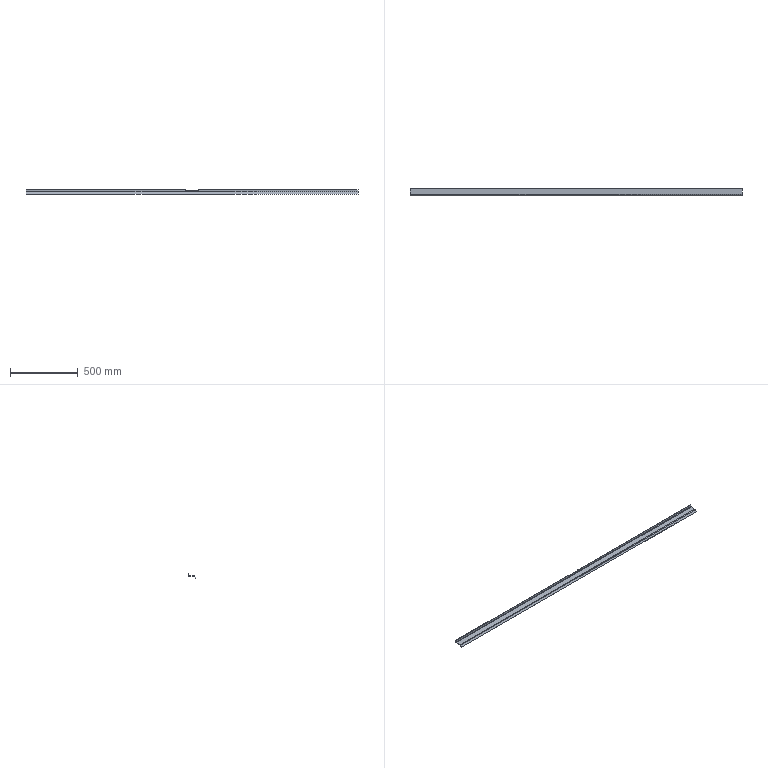Part | STEP file | Flat conveyor mechanism-CN2500x400-104-101_DefaultSM-FLAT-PATTERN | 1 solid | 26 faces | box 2450 x 58.268 x 35.821 mm | volume 594137 mm3 | plane 22 | cylinder 4 | commonest cylinder face diameters 6 x2 12 x2
STEP:
#1=CARTESIAN_POINT('',(-1225.,22.,17.));
#2=VERTEX_POINT('',#1);
#3=CARTESIAN_POINT('',(-50.,22.,17.));
#4=VERTEX_POINT('',#3);
#5=CARTESIAN_POINT('',(1225.,22.,17.));
#6=DIRECTION('',(1.,0.,0.));
#7=VECTOR('',#6,1000.);
#8=LINE('',#5,#7);
#9=EDGE_CURVE('',#2,#4,#8,.T.);
#10=ORIENTED_EDGE('',*,*,#9,.T.);
#11=CARTESIAN_POINT('',(-50.,25.,17.));
#12=VERTEX_POINT('',#11);
#13=CARTESIAN_POINT('',(-50.,25.,17.));
#14=DIRECTION('',(0.,1.,0.));
#15=VECTOR('',#14,1000.);
#16=LINE('',#13,#15);
#17=EDGE_CURVE('',#4,#12,#16,.T.);
#18=ORIENTED_EDGE('',*,*,#17,.T.);
#19=CARTESIAN_POINT('',(-1225.,25.,17.));
#20=VERTEX_POINT('',#19);
#21=CARTESIAN_POINT('',(0.,25.,17.));
#22=DIRECTION('',(1.,0.,0.));
#23=VECTOR('',#22,1000.);
#24=LINE('',#21,#23);
#25=EDGE_CURVE('',#20,#12,#24,.T.);
#26=ORIENTED_EDGE('',*,*,#25,.F.);
#27=CARTESIAN_POINT('',(-1225.,25.,17.));
#28=DIRECTION('',(0.,-1.,0.));
#29=VECTOR('',#28,1000.);
#30=LINE('',#27,#29);
#31=EDGE_CURVE('',#20,#2,#30,.T.);
#32=ORIENTED_EDGE('',*,*,#31,.T.);
#33=EDGE_LOOP('',(#10,#18,#26,#32));
#34=FACE_OUTER_BOUND('',#33,.T.);
#35=CARTESIAN_POINT('',(1225.,25.,17.));
#36=DIRECTION('',(0.,0.,-1.));
#37=DIRECTION('',(0.,1.,0.));
#38=AXIS2_PLACEMENT_3D('',#35,#36,#37);
#39=PLANE('',#38);
#40=ADVANCED_FACE('',(#34),#39,.F.);
#41=CARTESIAN_POINT('',(-1225.,19.,-3.));
#42=VERTEX_POINT('',#41);
#43=CARTESIAN_POINT('',(-1225.,-19.804,-3.));
#44=VERTEX_POINT('',#43);
#45=CARTESIAN_POINT('',(-1225.,25.,-3.));
#46=DIRECTION('',(0.,-1.,0.));
#47=VECTOR('',#46,1000.);
#48=LINE('',#45,#47);
#49=EDGE_CURVE('',#42,#44,#48,.T.);
#50=ORIENTED_EDGE('',*,*,#49,.T.);
#51=CARTESIAN_POINT('',(-1225.,-19.804,0.));
#52=VERTEX_POINT('',#51);
#53=CARTESIAN_POINT('',(-1225.,-19.804,-3.));
#54=DIRECTION('',(0.,0.,1.));
#55=VECTOR('',#54,1000.);
#56=LINE('',#53,#55);
#57=EDGE_CURVE('',#44,#52,#56,.T.);
#58=ORIENTED_EDGE('',*,*,#57,.T.);
#59=CARTESIAN_POINT('',(-1225.,19.,0.));
#60=VERTEX_POINT('',#59);
#61=CARTESIAN_POINT('',(-1225.,25.,0.));
#62=DIRECTION('',(0.,-1.,0.));
#63=VECTOR('',#62,1000.);
#64=LINE('',#61,#63);
#65=EDGE_CURVE('',#60,#52,#64,.T.);
#66=ORIENTED_EDGE('',*,*,#65,.F.);
#67=CARTESIAN_POINT('',(-1225.,19.,0.));
#68=DIRECTION('',(0.,0.,-1.));
#69=VECTOR('',#68,1000.);
#70=LINE('',#67,#69);
#71=EDGE_CURVE('',#60,#42,#70,.T.);
#72=ORIENTED_EDGE('',*,*,#71,.T.);
#73=EDGE_LOOP('',(#50,#58,#66,#72));
#74=FACE_OUTER_BOUND('',#73,.T.);
#75=CARTESIAN_POINT('',(-1225.,25.,-3.));
#76=DIRECTION('',(-1.,0.,0.));
#77=DIRECTION('',(0.,0.,1.));
#78=AXIS2_PLACEMENT_3D('',#75,#76,#77);
#79=PLANE('',#78);
#80=ADVANCED_FACE('',(#74),#79,.T.);
#81=CARTESIAN_POINT('',(1225.,-19.804,-3.));
#82=VERTEX_POINT('',#81);
#83=CARTESIAN_POINT('',(-1225.,-19.804,-3.));
#84=DIRECTION('',(1.,0.,0.));
#85=VECTOR('',#84,1000.);
#86=LINE('',#83,#85);
#87=EDGE_CURVE('',#44,#82,#86,.T.);
#88=ORIENTED_EDGE('',*,*,#87,.F.);
#89=ORIENTED_EDGE('',*,*,#49,.F.);
#90=CARTESIAN_POINT('',(1225.,19.,-3.));
#91=VERTEX_POINT('',#90);
#92=CARTESIAN_POINT('',(-1225.,19.,-3.));
#93=DIRECTION('',(1.,0.,0.));
#94=VECTOR('',#93,1000.);
#95=LINE('',#92,#94);
#96=EDGE_CURVE('',#42,#91,#95,.T.);
#97=ORIENTED_EDGE('',*,*,#96,.T.);
#98=CARTESIAN_POINT('',(1225.,25.,-3.));
#99=DIRECTION('',(0.,1.,0.));
#100=VECTOR('',#99,1000.);
#101=LINE('',#98,#100);
#102=EDGE_CURVE('',#82,#91,#101,.T.);
#103=ORIENTED_EDGE('',*,*,#102,.F.);
#104=EDGE_LOOP('',(#88,#89,#97,#103));
#105=FACE_OUTER_BOUND('',#104,.T.);
#106=CARTESIAN_POINT('',(0.,0.,-3.));
#107=DIRECTION('',(0.,0.,1.));
#108=DIRECTION('',(1.,0.,0.));
#109=AXIS2_PLACEMENT_3D('',#106,#107,#108);
#110=PLANE('',#109);
#111=ADVANCED_FACE('',(#105),#110,.F.);
#112=ORIENTED_EDGE('',*,*,#65,.T.);
#113=CARTESIAN_POINT('',(1225.,-19.804,0.));
#114=VERTEX_POINT('',#113);
#115=CARTESIAN_POINT('',(-1225.,-19.804,0.));
#116=DIRECTION('',(1.,0.,0.));
#117=VECTOR('',#116,1000.);
#118=LINE('',#115,#117);
#119=EDGE_CURVE('',#52,#114,#118,.T.);
#120=ORIENTED_EDGE('',*,*,#119,.T.);
#121=CARTESIAN_POINT('',(1225.,19.,0.));
#122=VERTEX_POINT('',#121);
#123=CARTESIAN_POINT('',(1225.,25.,0.));
#124=DIRECTION('',(0.,1.,0.));
#125=VECTOR('',#124,1000.);
#126=LINE('',#123,#125);
#127=EDGE_CURVE('',#114,#122,#126,.T.);
#128=ORIENTED_EDGE('',*,*,#127,.T.);
#129=CARTESIAN_POINT('',(-1225.,19.,0.));
#130=DIRECTION('',(1.,0.,0.));
#131=VECTOR('',#130,1000.);
#132=LINE('',#129,#131);
#133=EDGE_CURVE('',#60,#122,#132,.T.);
#134=ORIENTED_EDGE('',*,*,#133,.F.);
#135=EDGE_LOOP('',(#112,#120,#128,#134));
#136=FACE_OUTER_BOUND('',#135,.T.);
#137=CARTESIAN_POINT('',(0.,0.,0.));
#138=DIRECTION('',(0.,0.,1.));
#139=DIRECTION('',(1.,0.,0.));
#140=AXIS2_PLACEMENT_3D('',#137,#138,#139);
#141=PLANE('',#140);
#142=ADVANCED_FACE('',(#136),#141,.T.);
#143=CARTESIAN_POINT('',(1225.,-19.804,-3.));
#144=DIRECTION('',(0.,0.,1.));
#145=VECTOR('',#144,1000.);
#146=LINE('',#143,#145);
#147=EDGE_CURVE('',#82,#114,#146,.T.);
#148=ORIENTED_EDGE('',*,*,#147,.F.);
#149=ORIENTED_EDGE('',*,*,#102,.T.);
#150=CARTESIAN_POINT('',(1225.,19.,0.));
#151=DIRECTION('',(0.,0.,-1.));
#152=VECTOR('',#151,1000.);
#153=LINE('',#150,#152);
#154=EDGE_CURVE('',#122,#91,#153,.T.);
#155=ORIENTED_EDGE('',*,*,#154,.F.);
#156=ORIENTED_EDGE('',*,*,#127,.F.);
#157=EDGE_LOOP('',(#148,#149,#155,#156));
#158=FACE_OUTER_BOUND('',#157,.T.);
#159=CARTESIAN_POINT('',(1225.,25.,-3.));
#160=DIRECTION('',(1.,0.,0.));
#161=DIRECTION('',(0.,0.,-1.));
#162=AXIS2_PLACEMENT_3D('',#159,#160,#161);
#163=PLANE('',#162);
#164=ADVANCED_FACE('',(#158),#163,.T.);
#165=CARTESIAN_POINT('',(1225.,22.,3.));
#166=VERTEX_POINT('',#165);
#167=CARTESIAN_POINT('',(1225.,25.,3.));
#168=VERTEX_POINT('',#167);
#169=CARTESIAN_POINT('',(1225.,25.,3.));
#170=DIRECTION('',(0.,1.,0.));
#171=VECTOR('',#170,1000.);
#172=LINE('',#169,#171);
#173=EDGE_CURVE('',#166,#168,#172,.T.);
#174=ORIENTED_EDGE('',*,*,#173,.F.);
#175=CARTESIAN_POINT('',(1225.,19.,3.));
#176=DIRECTION('',(1.,0.,0.));
#177=DIRECTION('',(0.,0.,1.));
#178=AXIS2_PLACEMENT_3D('',#175,#176,#177);
#179=CIRCLE('',#178,3.);
#180=EDGE_CURVE('',#122,#166,#179,.T.);
#181=ORIENTED_EDGE('',*,*,#180,.F.);
#182=ORIENTED_EDGE('',*,*,#154,.T.);
#183=CARTESIAN_POINT('',(1225.,19.,3.));
#184=DIRECTION('',(1.,0.,0.));
#185=DIRECTION('',(0.,0.,1.));
#186=AXIS2_PLACEMENT_3D('',#183,#184,#185);
#187=CIRCLE('',#186,6.);
#188=EDGE_CURVE('',#91,#168,#187,.T.);
#189=ORIENTED_EDGE('',*,*,#188,.T.);
#190=EDGE_LOOP('',(#174,#181,#182,#189));
#191=FACE_OUTER_BOUND('',#190,.T.);
#192=CARTESIAN_POINT('',(1225.,19.,3.));
#193=DIRECTION('',(1.,0.,0.));
#194=DIRECTION('',(0.,0.,-1.));
#195=AXIS2_PLACEMENT_3D('',#192,#193,#194);
#196=PLANE('',#195);
#197=ADVANCED_FACE('',(#191),#196,.T.);
#198=CARTESIAN_POINT('',(-1225.,22.,3.));
#199=VERTEX_POINT('',#198);
#200=CARTESIAN_POINT('',(-1225.,19.,3.));
#201=DIRECTION('',(-1.,0.,0.));
#202=DIRECTION('',(0.,0.,1.));
#203=AXIS2_PLACEMENT_3D('',#200,#201,#202);
#204=CIRCLE('',#203,3.);
#205=EDGE_CURVE('',#199,#60,#204,.T.);
#206=ORIENTED_EDGE('',*,*,#205,.F.);
#207=CARTESIAN_POINT('',(-1225.,25.,3.));
#208=VERTEX_POINT('',#207);
#209=CARTESIAN_POINT('',(-1225.,22.,3.));
#210=DIRECTION('',(0.,1.,0.));
#211=VECTOR('',#210,1000.);
#212=LINE('',#209,#211);
#213=EDGE_CURVE('',#199,#208,#212,.T.);
#214=ORIENTED_EDGE('',*,*,#213,.T.);
#215=CARTESIAN_POINT('',(-1225.,19.,3.));
#216=DIRECTION('',(-1.,0.,0.));
#217=DIRECTION('',(0.,0.,1.));
#218=AXIS2_PLACEMENT_3D('',#215,#216,#217);
#219=CIRCLE('',#218,6.);
#220=EDGE_CURVE('',#208,#42,#219,.T.);
#221=ORIENTED_EDGE('',*,*,#220,.T.);
#222=ORIENTED_EDGE('',*,*,#71,.F.);
#223=EDGE_LOOP('',(#206,#214,#221,#222));
#224=FACE_OUTER_BOUND('',#223,.T.);
#225=CARTESIAN_POINT('',(-1225.,19.,3.));
#226=DIRECTION('',(1.,0.,0.));
#227=DIRECTION('',(0.,0.,-1.));
#228=AXIS2_PLACEMENT_3D('',#225,#226,#227);
#229=PLANE('',#228);
#230=ADVANCED_FACE('',(#224),#229,.F.);
#231=ORIENTED_EDGE('',*,*,#96,.F.);
#232=ORIENTED_EDGE('',*,*,#220,.F.);
#233=CARTESIAN_POINT('',(1225.,25.,3.));
#234=DIRECTION('',(1.,0.,0.));
#235=VECTOR('',#234,1000.);
#236=LINE('',#233,#235);
#237=EDGE_CURVE('',#208,#168,#236,.T.);
#238=ORIENTED_EDGE('',*,*,#237,.T.);
#239=ORIENTED_EDGE('',*,*,#188,.F.);
#240=EDGE_LOOP('',(#231,#232,#238,#239));
#241=FACE_OUTER_BOUND('',#240,.T.);
#242=CARTESIAN_POINT('',(-1225.,19.,3.));
#243=DIRECTION('',(-1.,0.,0.));
#244=DIRECTION('',(0.,1.,0.));
#245=AXIS2_PLACEMENT_3D('',#242,#243,#244);
#246=CYLINDRICAL_SURFACE('',#245,6.);
#247=ADVANCED_FACE('',(#241),#246,.T.);
#248=ORIENTED_EDGE('',*,*,#133,.T.);
#249=ORIENTED_EDGE('',*,*,#180,.T.);
#250=CARTESIAN_POINT('',(1225.,22.,3.));
#251=DIRECTION('',(-1.,0.,0.));
#252=VECTOR('',#251,1000.);
#253=LINE('',#250,#252);
#254=EDGE_CURVE('',#166,#199,#253,.T.);
#255=ORIENTED_EDGE('',*,*,#254,.T.);
#256=ORIENTED_EDGE('',*,*,#205,.T.);
#257=EDGE_LOOP('',(#248,#249,#255,#256));
#258=FACE_OUTER_BOUND('',#257,.T.);
#259=CARTESIAN_POINT('',(-1225.,19.,3.));
#260=DIRECTION('',(-1.,0.,0.));
#261=DIRECTION('',(0.,1.,0.));
#262=AXIS2_PLACEMENT_3D('',#259,#260,#261);
#263=CYLINDRICAL_SURFACE('',#262,3.);
#264=ADVANCED_FACE('',(#258),#263,.F.);
#265=ORIENTED_EDGE('',*,*,#213,.F.);
#266=CARTESIAN_POINT('',(-1225.,22.,17.));
#267=DIRECTION('',(0.,0.,1.));
#268=VECTOR('',#267,1000.);
#269=LINE('',#266,#268);
#270=EDGE_CURVE('',#199,#2,#269,.T.);
#271=ORIENTED_EDGE('',*,*,#270,.T.);
#272=ORIENTED_EDGE('',*,*,#31,.F.);
#273=CARTESIAN_POINT('',(-1225.,25.,0.));
#274=DIRECTION('',(0.,0.,1.));
#275=VECTOR('',#274,1000.);
#276=LINE('',#273,#275);
#277=EDGE_CURVE('',#208,#20,#276,.T.);
#278=ORIENTED_EDGE('',*,*,#277,.F.);
#279=EDGE_LOOP('',(#265,#271,#272,#278));
#280=FACE_OUTER_BOUND('',#279,.T.);
#281=CARTESIAN_POINT('',(-1225.,25.,17.));
#282=DIRECTION('',(1.,0.,0.));
#283=DIRECTION('',(0.,0.,-1.));
#284=AXIS2_PLACEMENT_3D('',#281,#282,#283);
#285=PLANE('',#284);
#286=ADVANCED_FACE('',(#280),#285,.F.);
#287=ORIENTED_EDGE('',*,*,#173,.T.);
#288=CARTESIAN_POINT('',(1225.,25.,17.));
#289=VERTEX_POINT('',#288);
#290=CARTESIAN_POINT('',(1225.,25.,0.));
#291=DIRECTION('',(0.,0.,-1.));
#292=VECTOR('',#291,1000.);
#293=LINE('',#290,#292);
#294=EDGE_CURVE('',#289,#168,#293,.T.);
#295=ORIENTED_EDGE('',*,*,#294,.F.);
#296=CARTESIAN_POINT('',(1225.,22.,17.));
#297=VERTEX_POINT('',#296);
#298=CARTESIAN_POINT('',(1225.,25.,17.));
#299=DIRECTION('',(0.,-1.,0.));
#300=VECTOR('',#299,1000.);
#301=LINE('',#298,#300);
#302=EDGE_CURVE('',#289,#297,#301,.T.);
#303=ORIENTED_EDGE('',*,*,#302,.T.);
#304=CARTESIAN_POINT('',(1225.,22.,0.));
#305=DIRECTION('',(0.,0.,-1.));
#306=VECTOR('',#305,1000.);
#307=LINE('',#304,#306);
#308=EDGE_CURVE('',#297,#166,#307,.T.);
#309=ORIENTED_EDGE('',*,*,#308,.T.);
#310=EDGE_LOOP('',(#287,#295,#303,#309));
#311=FACE_OUTER_BOUND('',#310,.T.);
#312=CARTESIAN_POINT('',(1225.,25.,0.));
#313=DIRECTION('',(-1.,0.,0.));
#314=DIRECTION('',(0.,0.,1.));
#315=AXIS2_PLACEMENT_3D('',#312,#313,#314);
#316=PLANE('',#315);
#317=ADVANCED_FACE('',(#311),#316,.F.);
#318=ORIENTED_EDGE('',*,*,#25,.T.);
#319=CARTESIAN_POINT('',(-50.,25.,10.));
#320=VERTEX_POINT('',#319);
#321=CARTESIAN_POINT('',(-50.,25.,10.));
#322=DIRECTION('',(0.,0.,1.));
#323=VECTOR('',#322,1000.);
#324=LINE('',#321,#323);
#325=EDGE_CURVE('',#320,#12,#324,.T.);
#326=ORIENTED_EDGE('',*,*,#325,.F.);
#327=CARTESIAN_POINT('',(50.,25.,10.));
#328=VERTEX_POINT('',#327);
#329=CARTESIAN_POINT('',(-50.,25.,10.));
#330=DIRECTION('',(-1.,0.,0.));
#331=VECTOR('',#330,1000.);
#332=LINE('',#329,#331);
#333=EDGE_CURVE('',#328,#320,#332,.T.);
#334=ORIENTED_EDGE('',*,*,#333,.F.);
#335=CARTESIAN_POINT('',(50.,25.,17.));
#336=VERTEX_POINT('',#335);
#337=CARTESIAN_POINT('',(50.,25.,10.));
#338=DIRECTION('',(0.,0.,-1.));
#339=VECTOR('',#338,1000.);
#340=LINE('',#337,#339);
#341=EDGE_CURVE('',#336,#328,#340,.T.);
#342=ORIENTED_EDGE('',*,*,#341,.F.);
#343=CARTESIAN_POINT('',(0.,25.,17.));
#344=DIRECTION('',(1.,0.,0.));
#345=VECTOR('',#344,1000.);
#346=LINE('',#343,#345);
#347=EDGE_CURVE('',#336,#289,#346,.T.);
#348=ORIENTED_EDGE('',*,*,#347,.T.);
#349=ORIENTED_EDGE('',*,*,#294,.T.);
#350=ORIENTED_EDGE('',*,*,#237,.F.);
#351=ORIENTED_EDGE('',*,*,#277,.T.);
#352=EDGE_LOOP('',(#318,#326,#334,#342,#348,#349,#350,#351));
#353=FACE_OUTER_BOUND('',#352,.T.);
#354=CARTESIAN_POINT('',(0.,25.,0.));
#355=DIRECTION('',(0.,-1.,0.));
#356=DIRECTION('',(0.,0.,-1.));
#357=AXIS2_PLACEMENT_3D('',#354,#355,#356);
#358=PLANE('',#357);
#359=ADVANCED_FACE('',(#353),#358,.F.);
#360=CARTESIAN_POINT('',(-50.,22.,10.));
#361=VERTEX_POINT('',#360);
#362=CARTESIAN_POINT('',(-50.,22.,0.));
#363=DIRECTION('',(0.,0.,-1.));
#364=VECTOR('',#363,1000.);
#365=LINE('',#362,#364);
#366=EDGE_CURVE('',#4,#361,#365,.T.);
#367=ORIENTED_EDGE('',*,*,#366,.F.);
#368=ORIENTED_EDGE('',*,*,#9,.F.);
#369=ORIENTED_EDGE('',*,*,#270,.F.);
#370=ORIENTED_EDGE('',*,*,#254,.F.);
#371=ORIENTED_EDGE('',*,*,#308,.F.);
#372=CARTESIAN_POINT('',(50.,22.,17.));
#373=VERTEX_POINT('',#372);
#374=CARTESIAN_POINT('',(1225.,22.,17.));
#375=DIRECTION('',(1.,0.,0.));
#376=VECTOR('',#375,1000.);
#377=LINE('',#374,#376);
#378=EDGE_CURVE('',#373,#297,#377,.T.);
#379=ORIENTED_EDGE('',*,*,#378,.F.);
#380=CARTESIAN_POINT('',(50.,22.,10.));
#381=VERTEX_POINT('',#380);
#382=CARTESIAN_POINT('',(50.,22.,0.));
#383=DIRECTION('',(0.,0.,1.));
#384=VECTOR('',#383,1000.);
#385=LINE('',#382,#384);
#386=EDGE_CURVE('',#381,#373,#385,.T.);
#387=ORIENTED_EDGE('',*,*,#386,.F.);
#388=CARTESIAN_POINT('',(0.,22.,10.));
#389=DIRECTION('',(1.,0.,0.));
#390=VECTOR('',#389,1000.);
#391=LINE('',#388,#390);
#392=EDGE_CURVE('',#361,#381,#391,.T.);
#393=ORIENTED_EDGE('',*,*,#392,.F.);
#394=EDGE_LOOP('',(#367,#368,#369,#370,#371,#379,#387,#393));
#395=FACE_OUTER_BOUND('',#394,.T.);
#396=CARTESIAN_POINT('',(0.,22.,0.));
#397=DIRECTION('',(0.,-1.,0.));
#398=DIRECTION('',(0.,0.,-1.));
#399=AXIS2_PLACEMENT_3D('',#396,#397,#398);
#400=PLANE('',#399);
#401=ADVANCED_FACE('',(#395),#400,.T.);
#402=ORIENTED_EDGE('',*,*,#347,.F.);
#403=CARTESIAN_POINT('',(50.,25.,17.));
#404=DIRECTION('',(0.,-1.,0.));
#405=VECTOR('',#404,1000.);
#406=LINE('',#403,#405);
#407=EDGE_CURVE('',#336,#373,#406,.T.);
#408=ORIENTED_EDGE('',*,*,#407,.T.);
#409=ORIENTED_EDGE('',*,*,#378,.T.);
#410=ORIENTED_EDGE('',*,*,#302,.F.);
#411=EDGE_LOOP('',(#402,#408,#409,#410));
#412=FACE_OUTER_BOUND('',#411,.T.);
#413=CARTESIAN_POINT('',(1225.,25.,17.));
#414=DIRECTION('',(0.,0.,-1.));
#415=DIRECTION('',(0.,1.,0.));
#416=AXIS2_PLACEMENT_3D('',#413,#414,#415);
#417=PLANE('',#416);
#418=ADVANCED_FACE('',(#412),#417,.F.);
#419=CARTESIAN_POINT('',(1225.,-22.402,-4.5));
#420=VERTEX_POINT('',#419);
#421=CARTESIAN_POINT('',(1225.,-25.,-3.));
#422=VERTEX_POINT('',#421);
#423=CARTESIAN_POINT('',(1225.,-25.,-3.));
#424=DIRECTION('',(0.,-0.866,0.5));
#425=VECTOR('',#424,1000.);
#426=LINE('',#423,#425);
#427=EDGE_CURVE('',#420,#422,#426,.T.);
#428=ORIENTED_EDGE('',*,*,#427,.F.);
#429=CARTESIAN_POINT('',(1225.,-19.804,-6.));
#430=DIRECTION('',(1.,0.,0.));
#431=DIRECTION('',(0.,0.,1.));
#432=AXIS2_PLACEMENT_3D('',#429,#430,#431);
#433=CIRCLE('',#432,3.);
#434=EDGE_CURVE('',#82,#420,#433,.T.);
#435=ORIENTED_EDGE('',*,*,#434,.F.);
#436=ORIENTED_EDGE('',*,*,#147,.T.);
#437=CARTESIAN_POINT('',(1225.,-19.804,-6.));
#438=DIRECTION('',(1.,0.,0.));
#439=DIRECTION('',(0.,0.,1.));
#440=AXIS2_PLACEMENT_3D('',#437,#438,#439);
#441=CIRCLE('',#440,6.);
#442=EDGE_CURVE('',#114,#422,#441,.T.);
#443=ORIENTED_EDGE('',*,*,#442,.T.);
#444=EDGE_LOOP('',(#428,#435,#436,#443));
#445=FACE_OUTER_BOUND('',#444,.T.);
#446=CARTESIAN_POINT('',(1225.,-19.804,-6.));
#447=DIRECTION('',(1.,0.,0.));
#448=DIRECTION('',(0.,0.,-1.));
#449=AXIS2_PLACEMENT_3D('',#446,#447,#448);
#450=PLANE('',#449);
#451=ADVANCED_FACE('',(#445),#450,.T.);
#452=CARTESIAN_POINT('',(-1225.,-22.402,-4.5));
#453=VERTEX_POINT('',#452);
#454=CARTESIAN_POINT('',(-1225.,-19.804,-6.));
#455=DIRECTION('',(-1.,0.,0.));
#456=DIRECTION('',(0.,0.,1.));
#457=AXIS2_PLACEMENT_3D('',#454,#455,#456);
#458=CIRCLE('',#457,3.);
#459=EDGE_CURVE('',#453,#44,#458,.T.);
#460=ORIENTED_EDGE('',*,*,#459,.F.);
#461=CARTESIAN_POINT('',(-1225.,-25.,-3.));
#462=VERTEX_POINT('',#461);
#463=CARTESIAN_POINT('',(-1225.,-22.402,-4.5));
#464=DIRECTION('',(0.,-0.866,0.5));
#465=VECTOR('',#464,1000.);
#466=LINE('',#463,#465);
#467=EDGE_CURVE('',#453,#462,#466,.T.);
#468=ORIENTED_EDGE('',*,*,#467,.T.);
#469=CARTESIAN_POINT('',(-1225.,-19.804,-6.));
#470=DIRECTION('',(-1.,0.,0.));
#471=DIRECTION('',(0.,0.,1.));
#472=AXIS2_PLACEMENT_3D('',#469,#470,#471);
#473=CIRCLE('',#472,6.);
#474=EDGE_CURVE('',#462,#52,#473,.T.);
#475=ORIENTED_EDGE('',*,*,#474,.T.);
#476=ORIENTED_EDGE('',*,*,#57,.F.);
#477=EDGE_LOOP('',(#460,#468,#475,#476));
#478=FACE_OUTER_BOUND('',#477,.T.);
#479=CARTESIAN_POINT('',(-1225.,-19.804,-6.));
#480=DIRECTION('',(1.,0.,0.));
#481=DIRECTION('',(0.,0.,-1.));
#482=AXIS2_PLACEMENT_3D('',#479,#480,#481);
#483=PLANE('',#482);
#484=ADVANCED_FACE('',(#478),#483,.F.);
#485=ORIENTED_EDGE('',*,*,#119,.F.);
#486=ORIENTED_EDGE('',*,*,#474,.F.);
#487=CARTESIAN_POINT('',(0.,-25.,-3.));
#488=DIRECTION('',(-1.,0.,0.));
#489=VECTOR('',#488,1000.);
#490=LINE('',#487,#489);
#491=EDGE_CURVE('',#422,#462,#490,.T.);
#492=ORIENTED_EDGE('',*,*,#491,.F.);
#493=ORIENTED_EDGE('',*,*,#442,.F.);
#494=EDGE_LOOP('',(#485,#486,#492,#493));
#495=FACE_OUTER_BOUND('',#494,.T.);
#496=CARTESIAN_POINT('',(-1225.,-19.804,-6.));
#497=DIRECTION('',(-1.,0.,0.));
#498=DIRECTION('',(0.,-0.866,0.5));
#499=AXIS2_PLACEMENT_3D('',#496,#497,#498);
#500=CYLINDRICAL_SURFACE('',#499,6.);
#501=ADVANCED_FACE('',(#495),#500,.T.);
#502=ORIENTED_EDGE('',*,*,#87,.T.);
#503=ORIENTED_EDGE('',*,*,#434,.T.);
#504=CARTESIAN_POINT('',(1225.,-22.402,-4.5));
#505=DIRECTION('',(-1.,0.,0.));
#506=VECTOR('',#505,1000.);
#507=LINE('',#504,#506);
#508=EDGE_CURVE('',#420,#453,#507,.T.);
#509=ORIENTED_EDGE('',*,*,#508,.T.);
#510=ORIENTED_EDGE('',*,*,#459,.T.);
#511=EDGE_LOOP('',(#502,#503,#509,#510));
#512=FACE_OUTER_BOUND('',#511,.T.);
#513=CARTESIAN_POINT('',(-1225.,-19.804,-6.));
#514=DIRECTION('',(-1.,0.,0.));
#515=DIRECTION('',(0.,-0.866,0.5));
#516=AXIS2_PLACEMENT_3D('',#513,#514,#515);
#517=CYLINDRICAL_SURFACE('',#516,3.);
#518=ADVANCED_FACE('',(#512),#517,.F.);
#519=CARTESIAN_POINT('',(-1225.,-33.268,-17.321));
#520=VERTEX_POINT('',#519);
#521=CARTESIAN_POINT('',(-1225.,-24.134,-1.5));
#522=DIRECTION('',(0.,0.5,0.866));
#523=VECTOR('',#522,1000.);
#524=LINE('',#521,#523);
#525=EDGE_CURVE('',#520,#462,#524,.T.);
#526=ORIENTED_EDGE('',*,*,#525,.T.);
#527=ORIENTED_EDGE('',*,*,#467,.F.);
#528=CARTESIAN_POINT('',(-1225.,-30.67,-18.821));
#529=VERTEX_POINT('',#528);
#530=CARTESIAN_POINT('',(-1225.,-13.987,10.075));
#531=DIRECTION('',(0.,0.5,0.866));
#532=VECTOR('',#531,1000.);
#533=LINE('',#530,#532);
#534=EDGE_CURVE('',#529,#453,#533,.T.);
#535=ORIENTED_EDGE('',*,*,#534,.F.);
#536=CARTESIAN_POINT('',(-1225.,-33.268,-17.321));
#537=DIRECTION('',(0.,0.866,-0.5));
#538=VECTOR('',#537,1000.);
#539=LINE('',#536,#538);
#540=EDGE_CURVE('',#520,#529,#539,.T.);
#541=ORIENTED_EDGE('',*,*,#540,.F.);
#542=EDGE_LOOP('',(#526,#527,#535,#541));
#543=FACE_OUTER_BOUND('',#542,.T.);
#544=CARTESIAN_POINT('',(-1225.,-24.134,-1.5));
#545=DIRECTION('',(-1.,0.,0.));
#546=DIRECTION('',(0.,0.,1.));
#547=AXIS2_PLACEMENT_3D('',#544,#545,#546);
#548=PLANE('',#547);
#549=ADVANCED_FACE('',(#543),#548,.T.);
#550=CARTESIAN_POINT('',(1225.,-30.67,-18.821));
#551=VERTEX_POINT('',#550);
#552=CARTESIAN_POINT('',(1225.,-13.987,10.075));
#553=DIRECTION('',(0.,-0.5,-0.866));
#554=VECTOR('',#553,1000.);
#555=LINE('',#552,#554);
#556=EDGE_CURVE('',#420,#551,#555,.T.);
#557=ORIENTED_EDGE('',*,*,#556,.F.);
#558=ORIENTED_EDGE('',*,*,#427,.T.);
#559=CARTESIAN_POINT('',(1225.,-33.268,-17.321));
#560=VERTEX_POINT('',#559);
#561=CARTESIAN_POINT('',(1225.,-33.268,-17.321));
#562=DIRECTION('',(0.,-0.5,-0.866));
#563=VECTOR('',#562,1000.);
#564=LINE('',#561,#563);
#565=EDGE_CURVE('',#422,#560,#564,.T.);
#566=ORIENTED_EDGE('',*,*,#565,.T.);
#567=CARTESIAN_POINT('',(1225.,-33.268,-17.321));
#568=DIRECTION('',(0.,0.866,-0.5));
#569=VECTOR('',#568,1000.);
#570=LINE('',#567,#569);
#571=EDGE_CURVE('',#560,#551,#570,.T.);
#572=ORIENTED_EDGE('',*,*,#571,.T.);
#573=EDGE_LOOP('',(#557,#558,#566,#572));
#574=FACE_OUTER_BOUND('',#573,.T.);
#575=CARTESIAN_POINT('',(1225.,-33.268,-17.321));
#576=DIRECTION('',(1.,0.,0.));
#577=DIRECTION('',(0.,0.,-1.));
#578=AXIS2_PLACEMENT_3D('',#575,#576,#577);
#579=PLANE('',#578);
#580=ADVANCED_FACE('',(#574),#579,.T.);
#581=ORIENTED_EDGE('',*,*,#565,.F.);
#582=ORIENTED_EDGE('',*,*,#491,.T.);
#583=ORIENTED_EDGE('',*,*,#525,.F.);
#584=CARTESIAN_POINT('',(-1225.,-33.268,-17.321));
#585=DIRECTION('',(-1.,0.,0.));
#586=VECTOR('',#585,1000.);
#587=LINE('',#584,#586);
#588=EDGE_CURVE('',#560,#520,#587,.T.);
#589=ORIENTED_EDGE('',*,*,#588,.F.);
#590=EDGE_LOOP('',(#581,#582,#583,#589));
#591=FACE_OUTER_BOUND('',#590,.T.);
#592=CARTESIAN_POINT('',(0.,-16.585,11.575));
#593=DIRECTION('',(0.,-0.866,0.5));
#594=DIRECTION('',(0.,-0.5,-0.866));
#595=AXIS2_PLACEMENT_3D('',#592,#593,#594);
#596=PLANE('',#595);
#597=ADVANCED_FACE('',(#591),#596,.T.);
#598=ORIENTED_EDGE('',*,*,#508,.F.);
#599=ORIENTED_EDGE('',*,*,#556,.T.);
#600=CARTESIAN_POINT('',(0.,-30.67,-18.821));
#601=DIRECTION('',(-1.,0.,0.));
#602=VECTOR('',#601,1000.);
#603=LINE('',#600,#602);
#604=EDGE_CURVE('',#551,#529,#603,.T.);
#605=ORIENTED_EDGE('',*,*,#604,.T.);
#606=ORIENTED_EDGE('',*,*,#534,.T.);
#607=EDGE_LOOP('',(#598,#599,#605,#606));
#608=FACE_OUTER_BOUND('',#607,.T.);
#609=CARTESIAN_POINT('',(0.,-13.987,10.075));
#610=DIRECTION('',(0.,-0.866,0.5));
#611=DIRECTION('',(0.,-0.5,-0.866));
#612=AXIS2_PLACEMENT_3D('',#609,#610,#611);
#613=PLANE('',#612);
#614=ADVANCED_FACE('',(#608),#613,.F.);
#615=ORIENTED_EDGE('',*,*,#604,.F.);
#616=ORIENTED_EDGE('',*,*,#571,.F.);
#617=ORIENTED_EDGE('',*,*,#588,.T.);
#618=ORIENTED_EDGE('',*,*,#540,.T.);
#619=EDGE_LOOP('',(#615,#616,#617,#618));
#620=FACE_OUTER_BOUND('',#619,.T.);
#621=CARTESIAN_POINT('',(-1225.,-33.268,-17.321));
#622=DIRECTION('',(0.,-0.5,-0.866));
#623=DIRECTION('',(0.,0.866,-0.5));
#624=AXIS2_PLACEMENT_3D('',#621,#622,#623);
#625=PLANE('',#624);
#626=ADVANCED_FACE('',(#620),#625,.T.);
#627=ORIENTED_EDGE('',*,*,#366,.T.);
#628=CARTESIAN_POINT('',(-50.,15.,10.));
#629=DIRECTION('',(0.,1.,0.));
#630=VECTOR('',#629,1000.);
#631=LINE('',#628,#630);
#632=EDGE_CURVE('',#361,#320,#631,.T.);
#633=ORIENTED_EDGE('',*,*,#632,.T.);
#634=ORIENTED_EDGE('',*,*,#325,.T.);
#635=ORIENTED_EDGE('',*,*,#17,.F.);
#636=EDGE_LOOP('',(#627,#633,#634,#635));
#637=FACE_OUTER_BOUND('',#636,.T.);
#638=CARTESIAN_POINT('',(-50.,15.,10.));
#639=DIRECTION('',(-1.,0.,0.));
#640=DIRECTION('',(0.,0.,1.));
#641=AXIS2_PLACEMENT_3D('',#638,#639,#640);
#642=PLANE('',#641);
#643=ADVANCED_FACE('',(#637),#642,.F.);
#644=ORIENTED_EDGE('',*,*,#392,.T.);
#645=CARTESIAN_POINT('',(50.,15.,10.));
#646=DIRECTION('',(0.,1.,0.));
#647=VECTOR('',#646,1000.);
#648=LINE('',#645,#647);
#649=EDGE_CURVE('',#381,#328,#648,.T.);
#650=ORIENTED_EDGE('',*,*,#649,.T.);
#651=ORIENTED_EDGE('',*,*,#333,.T.);
#652=ORIENTED_EDGE('',*,*,#632,.F.);
#653=EDGE_LOOP('',(#644,#650,#651,#652));
#654=FACE_OUTER_BOUND('',#653,.T.);
#655=CARTESIAN_POINT('',(-50.,15.,10.));
#656=DIRECTION('',(0.,0.,-1.));
#657=DIRECTION('',(0.,1.,0.));
#658=AXIS2_PLACEMENT_3D('',#655,#656,#657);
#659=PLANE('',#658);
#660=ADVANCED_FACE('',(#654),#659,.F.);
#661=ORIENTED_EDGE('',*,*,#386,.T.);
#662=ORIENTED_EDGE('',*,*,#407,.F.);
#663=ORIENTED_EDGE('',*,*,#341,.T.);
#664=ORIENTED_EDGE('',*,*,#649,.F.);
#665=EDGE_LOOP('',(#661,#662,#663,#664));
#666=FACE_OUTER_BOUND('',#665,.T.);
#667=CARTESIAN_POINT('',(50.,15.,10.));
#668=DIRECTION('',(1.,0.,0.));
#669=DIRECTION('',(0.,0.,-1.));
#670=AXIS2_PLACEMENT_3D('',#667,#668,#669);
#671=PLANE('',#670);
#672=ADVANCED_FACE('',(#666),#671,.F.);
#673=CLOSED_SHELL('',(#40,#80,#111,#142,#164,#197,#230,#247,#264,#286,#317,#359,#401,#418,#451,#484,#501,#518,#549,#580,#597,#614,#626,#643,#660,#672));
#674=MANIFOLD_SOLID_BREP('',#673);
#675=CARTESIAN_POINT('',(0.,0.,0.));
#676=DIRECTION('',(0.,0.,1.));
#677=DIRECTION('',(1.,0.,0.));
#678=AXIS2_PLACEMENT_3D('',#675,#676,#677);
#679=(LENGTH_UNIT()NAMED_UNIT(*)SI_UNIT(.MILLI.,.METRE.));
#680=UNCERTAINTY_MEASURE_WITH_UNIT(LENGTH_MEASURE(0.00001),#679,'','');
#681=(NAMED_UNIT(*)PLANE_ANGLE_UNIT()SI_UNIT($,.RADIAN.));
#682=(NAMED_UNIT(*)SI_UNIT($,.STERADIAN.)SOLID_ANGLE_UNIT());
#683=(GEOMETRIC_REPRESENTATION_CONTEXT(3)GLOBAL_UNCERTAINTY_ASSIGNED_CONTEXT((#680))GLOBAL_UNIT_ASSIGNED_CONTEXT((#679,#681,#682))REPRESENTATION_CONTEXT('',''));
#684=ADVANCED_BREP_SHAPE_REPRESENTATION('',(#674,#678),#683);